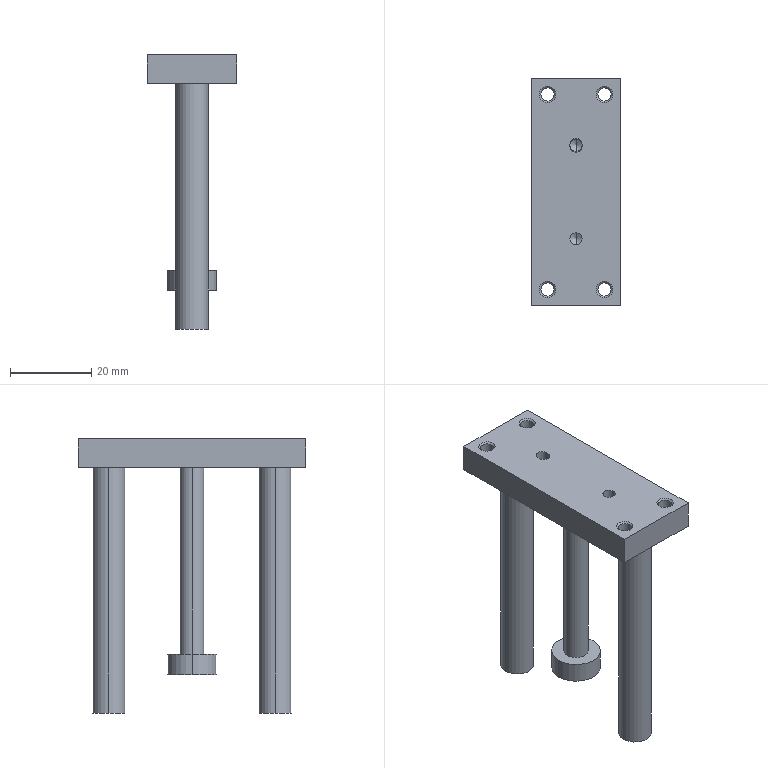Part | SolidWorks | features BaseBody 1 | 1 solid | 56 faces | box 22 x 56 x 67.5 mm | volume 16241 mm3 | cylinder 22 | cone 20 | plane 14 | commonest cylinder face diameters 3.242 x8 3 x6 8 x4 6 x2 12 x2